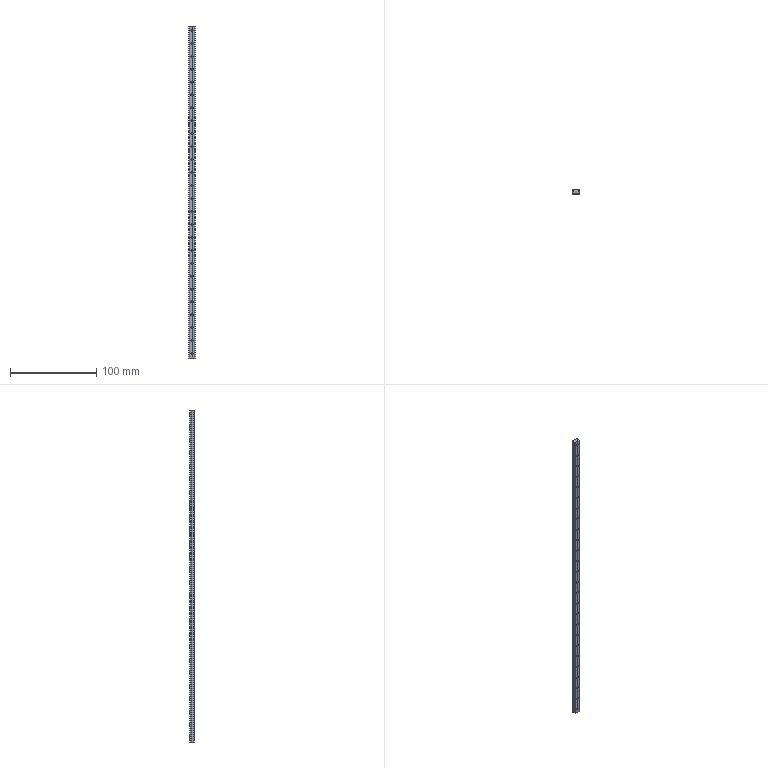Part | STEP file | MGN7C-rail L385 | 1 solid | 173 faces | box 7 x 4.8 x 385 mm | volume 11143 mm3 | cylinder 134 | plane 39 | commonest cylinder face diameters 2.4 x52 4.2 x52 0.6 x27 1.4 x3